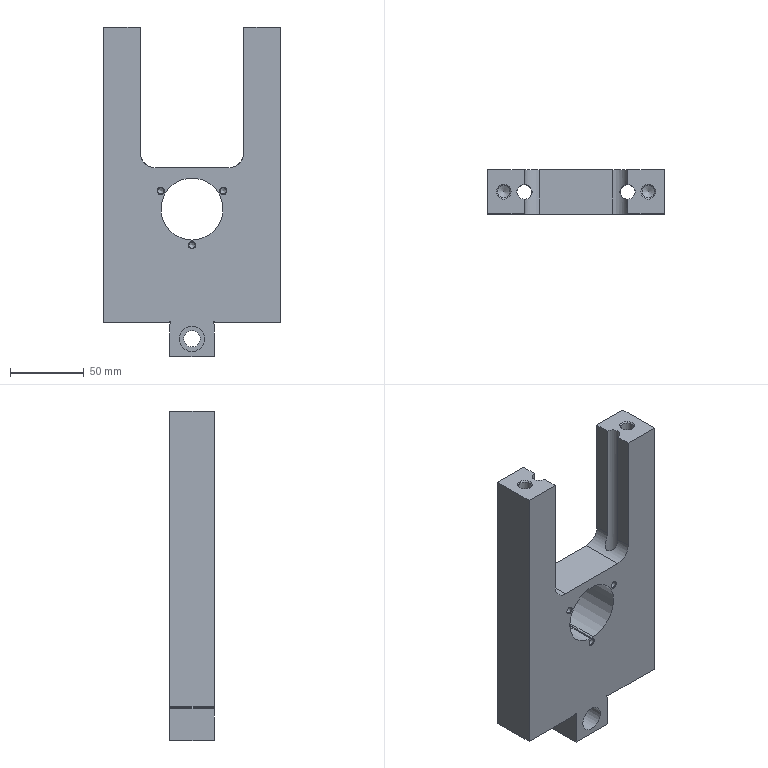Part | STEP file | YBQDJ-YB-2 | 1 solid | 60 faces | box 120 x 30 x 223 mm | volume 466414 mm3 | cylinder 29 | plane 17 | cone 14 | commonest cylinder face diameters 4 x10 1 x5 8.5 x4 4.2 x3 10.06 x2 20 x2